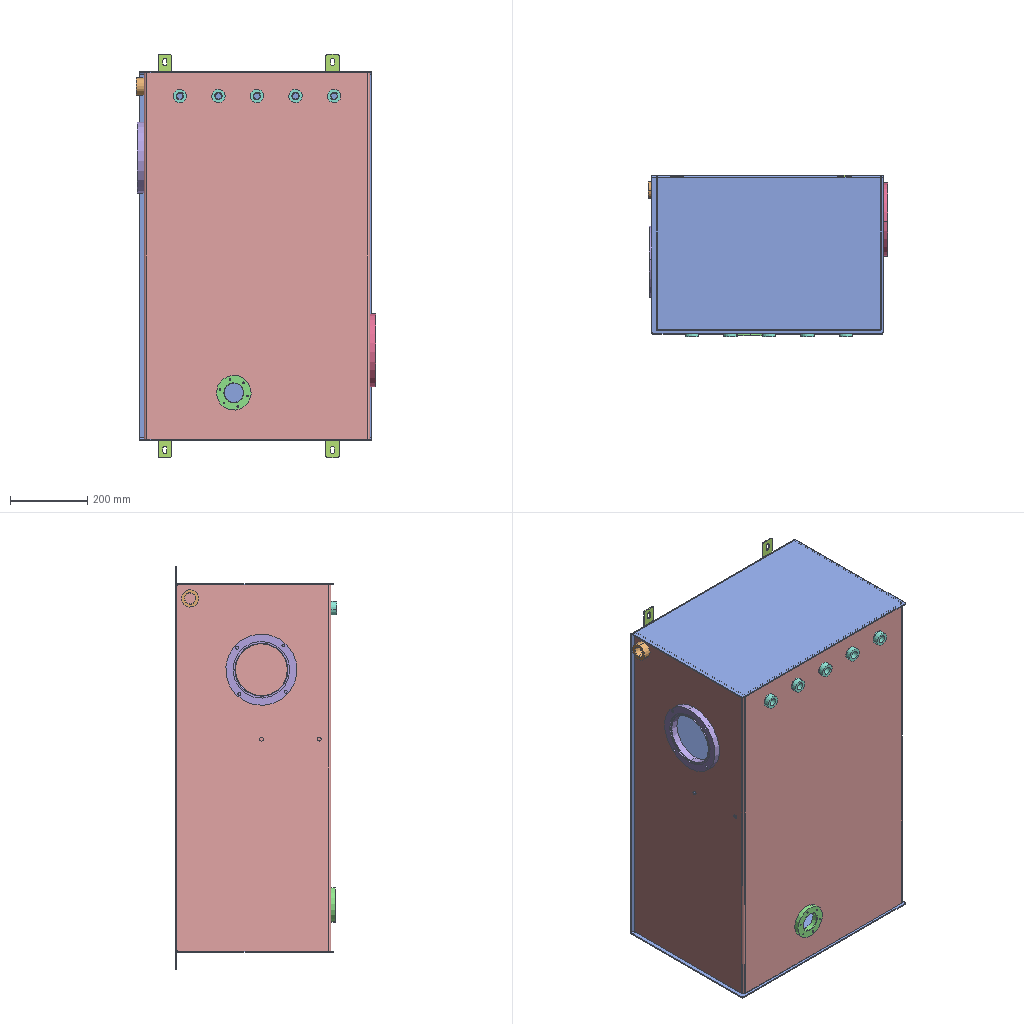Assembly | SolidWorks | 10 different items | 25 placed | box 621 x 418 x 1046 mm
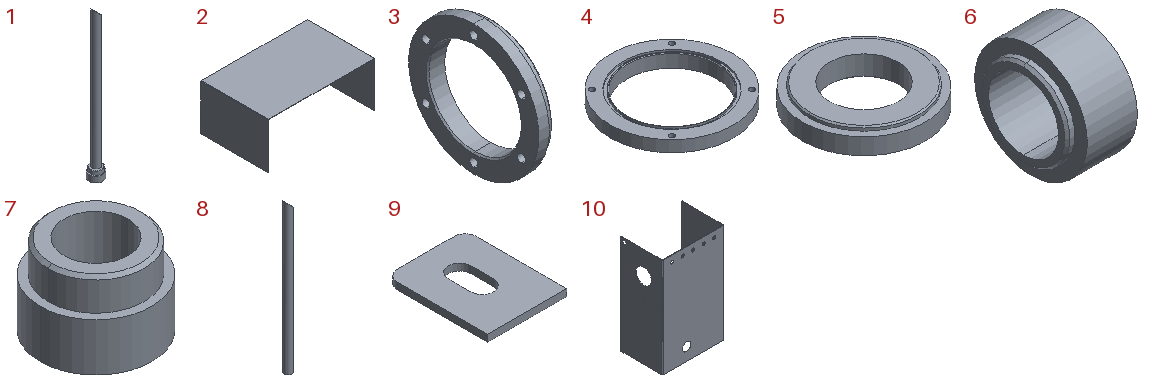Parts list (item | name | quantity | parent item | size | volume | features):
1 | (subassembly) | x5 | - | 35 x 35 x 370 mm | 31813 mm3 | features CompositeCurve 2
2 | - | x1 | - | 956 x 600 x 410 mm | 3179024 mm3 | features FlatPattern 1, ICE 1, SMBaseFlange 1, SheetMetal 1
3 | - | x1 | - | 25 x 190 x 190 mm | 309030 mm3 | features ICE 2, Chamfer 1, Extrusion 1
4 | - | x1 | - | 185 x 185 x 20 mm | 215691 mm3 | features ICE 3, Chamfer 1, Extrusion 1
5 | - | x1 | - | 90 x 90 x 15 mm | 60934 mm3 | features ICE 2, Chamfer 1, Extrusion 1
6 | - | x1 | - | 23 x 45 x 45 mm | 20434 mm3 | features Chamfer 1, Extrusion 1, ICE 1
7 | - | x5 | in 1 | 35 x 35 x 25 mm | 13600 mm3 | features Chamfer 1, Extrusion 1, ICE 1
8 | - | x5 | in 1 | 18 x 18 x 350 mm | 18212 mm3 | features Extrusion 1, ICE 1
9 | - | x4 | - | 35 x 45 x 3 mm | 4157 mm3 | features Extrusion 1
10 | - | x1 | - | 586 x 400 x 950 mm | 3763524 mm3 | features ICE 4, FlatPattern 1, SMBaseFlange 1, SheetMetal 1
Mates (type | each side: item.copy, entity, surface, feature):
In the top assembly
Coincident | 10.1 face plane Base-Flange1 | 2.1 face plane Base-Flange1 | 2 times
DistanceDim | 2.1 face plane Base-Flange1 | 10.1 face plane Base-Flange1
Coincident | 2.1 face plane Base-Flange1 | 9.1 face plane Boss-Extrude1 | 2 times
DistanceDim | 9.1 face plane Boss-Extrude1 | 2.1 face plane Base-Flange1
Coincident | 9.2 face plane Boss-Extrude1 | 9.3 face plane Boss-Extrude1 | 2 times
Coincident | 9.3 face plane Boss-Extrude1 | 9.4 face plane Boss-Extrude1 | 2 times
Coincident | 9.1 face plane Boss-Extrude1 | 9.4 face plane Boss-Extrude1 | 2 times
Coincident | 9.1 face plane Boss-Extrude1 | 9.2 face plane Boss-Extrude1
DistanceDim | 9.1 face plane Boss-Extrude1 | 9.2 face plane Boss-Extrude1
Coincident | 2.1 face plane Base-Flange1 | 9.4 face plane Boss-Extrude1
Coincident | 10.1 face plane Base-Flange1 | 7.1 face plane Cut-Extrude1
Concentric | 10.1 edge | 7.1 edge
Coincident | 7.1 face plane Boss-Extrude1 | 7.2 face plane Boss-Extrude1
Coincident | 7.3 face plane Boss-Extrude1 | 7.2 face plane Boss-Extrude1
Coincident | 7.3 face plane Boss-Extrude1 | 7.4 face plane Boss-Extrude1
Coincident | 7.4 face plane Boss-Extrude1 | 7.5 face plane Boss-Extrude1
Concentric | 10.1 edge | 7.5 edge
Concentric | 10.1 edge | 7.4 edge
Concentric | 10.1 edge | 7.3 edge
Concentric | 10.1 edge | 7.2 edge
Concentric | 10.1 edge | 6.1 edge
Coincident | 10.1 face plane Base-Flange1 | 6.1 face plane Cut-Extrude1
Coincident | 10.1 face plane Base-Flange1 | 4.1 face plane Cut-Extrude3
Concentric | 10.1 edge | 4.1 edge
Coincident | 10.1 face plane Base-Flange1 | 5.1 face plane Cut-Extrude1
Concentric | 10.1 edge | 5.1 edge
Coincident | 10.1 face plane Base-Flange1 | 3.1 face plane Cut-Extrude1
Concentric | 10.1 edge | 3.1 edge
In subassembly 1
Concentric | 8.1 edge | 7.6 edge
DistanceDim | 8.1 face plane Boss-Extrude1 | 7.6 face plane Boss-Extrude1